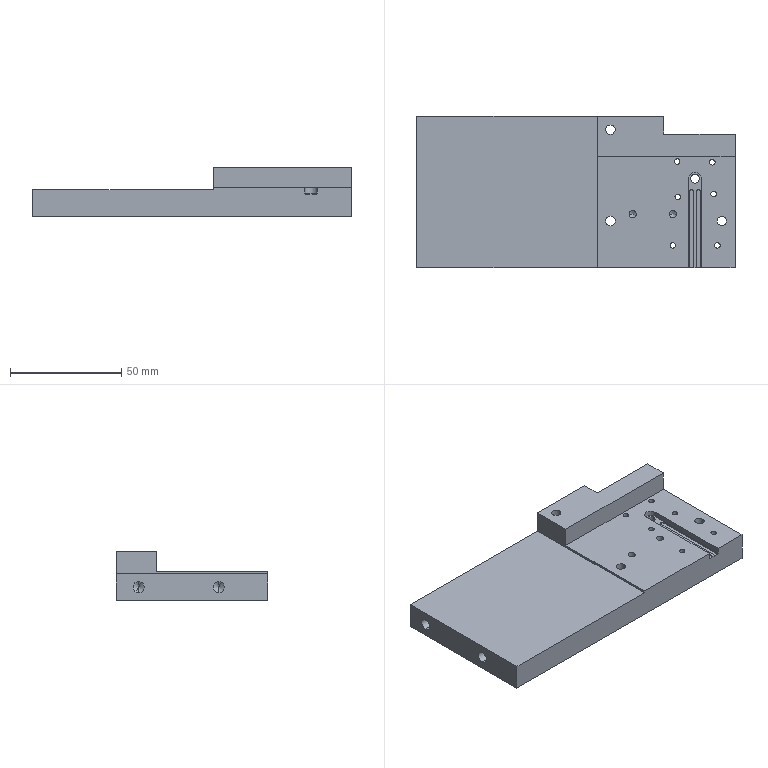Part | STEP file | BU-B01 | 1 solid | 63 faces | box 143 x 68 x 22 mm | volume 122394 mm3 | cylinder 33 | plane 22 | cone 8 | commonest cylinder face diameters 2.5 x12 4.2 x6 3.3 x4 5 x4 2 x2 4 x2